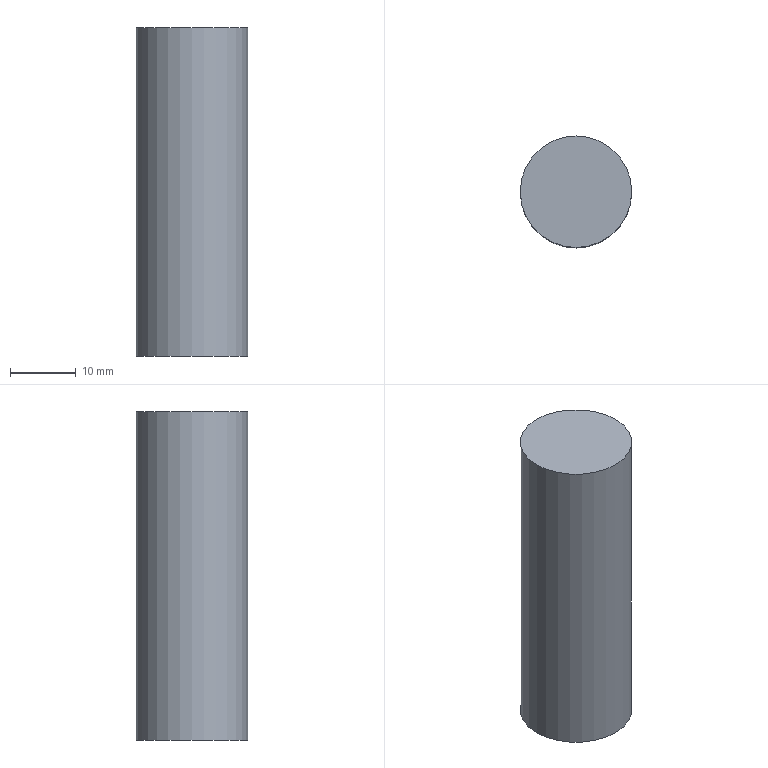Part | NX | features BREP 2 | 2 solids | 7 faces | box 17 x 17 x 50 mm | volume 12091 mm3 | plane 4 | cylinder 3 | commonest cylinder face diameters 6 x1 15 x1 17 x1
STEP:
#1=CARTESIAN_POINT('',(8.5,0.,97.));
#2=VERTEX_POINT('',#1);
#3=CARTESIAN_POINT('',(0.,0.,97.));
#4=DIRECTION('',(0.,0.,1.));
#5=DIRECTION('',(1.,0.,0.));
#6=AXIS2_PLACEMENT_3D('',#3,#4,#5);
#7=CIRCLE('',#6,8.5);
#8=EDGE_CURVE('',#2,#2,#7,.T.);
#9=ORIENTED_EDGE('',*,*,#8,.F.);
#10=EDGE_LOOP('',(#9));
#11=FACE_BOUND('',#10,.T.);
#12=CARTESIAN_POINT('',(8.5,0.,47.));
#13=VERTEX_POINT('',#12);
#14=CARTESIAN_POINT('',(0.,0.,47.));
#15=DIRECTION('',(0.,0.,1.));
#16=DIRECTION('',(1.,0.,0.));
#17=AXIS2_PLACEMENT_3D('',#14,#15,#16);
#18=CIRCLE('',#17,8.5);
#19=EDGE_CURVE('',#13,#13,#18,.T.);
#20=ORIENTED_EDGE('',*,*,#19,.T.);
#21=EDGE_LOOP('',(#20));
#22=FACE_BOUND('',#21,.T.);
#23=CARTESIAN_POINT('',(0.,0.,97.));
#24=DIRECTION('',(0.,0.,-1.));
#25=DIRECTION('',(1.,0.,0.));
#26=AXIS2_PLACEMENT_3D('',#23,#24,#25);
#27=CYLINDRICAL_SURFACE('',#26,8.5);
#28=ADVANCED_FACE('',(#11,#22),#27,.T.);
#29=ORIENTED_EDGE('',*,*,#8,.T.);
#30=EDGE_LOOP('',(#29));
#31=FACE_BOUND('',#30,.T.);
#32=CARTESIAN_POINT('',(0.,0.,97.));
#33=DIRECTION('',(0.,0.,1.));
#34=DIRECTION('',(-1.,0.,0.));
#35=AXIS2_PLACEMENT_3D('',#32,#33,#34);
#36=PLANE('',#35);
#37=ADVANCED_FACE('',(#31),#36,.T.);
#38=ORIENTED_EDGE('',*,*,#19,.F.);
#39=EDGE_LOOP('',(#38));
#40=FACE_BOUND('',#39,.T.);
#41=CARTESIAN_POINT('',(0.,0.,47.));
#42=DIRECTION('',(0.,0.,1.));
#43=DIRECTION('',(-1.,0.,0.));
#44=AXIS2_PLACEMENT_3D('',#41,#42,#43);
#45=PLANE('',#44);
#46=ADVANCED_FACE('',(#40),#45,.F.);
#47=CLOSED_SHELL('',(#28,#37,#46));
#48=MANIFOLD_SOLID_BREP('',#47);
#49=CARTESIAN_POINT('',(7.5,0.,60.));
#50=VERTEX_POINT('',#49);
#51=CARTESIAN_POINT('',(0.,0.,60.));
#52=DIRECTION('',(0.,0.,1.));
#53=DIRECTION('',(1.,0.,0.));
#54=AXIS2_PLACEMENT_3D('',#51,#52,#53);
#55=CIRCLE('',#54,7.5);
#56=EDGE_CURVE('',#50,#50,#55,.T.);
#57=ORIENTED_EDGE('',*,*,#56,.F.);
#58=EDGE_LOOP('',(#57));
#59=FACE_BOUND('',#58,.T.);
#60=CARTESIAN_POINT('',(7.5,0.,55.));
#61=VERTEX_POINT('',#60);
#62=CARTESIAN_POINT('',(0.,0.,55.));
#63=DIRECTION('',(0.,0.,1.));
#64=DIRECTION('',(1.,0.,0.));
#65=AXIS2_PLACEMENT_3D('',#62,#63,#64);
#66=CIRCLE('',#65,7.5);
#67=EDGE_CURVE('',#61,#61,#66,.T.);
#68=ORIENTED_EDGE('',*,*,#67,.T.);
#69=EDGE_LOOP('',(#68));
#70=FACE_BOUND('',#69,.T.);
#71=CARTESIAN_POINT('',(0.,0.,60.));
#72=DIRECTION('',(0.,0.,-1.));
#73=DIRECTION('',(1.,0.,0.));
#74=AXIS2_PLACEMENT_3D('',#71,#72,#73);
#75=CYLINDRICAL_SURFACE('',#74,7.5);
#76=ADVANCED_FACE('',(#59,#70),#75,.T.);
#77=CARTESIAN_POINT('',(3.,0.,60.));
#78=VERTEX_POINT('',#77);
#79=CARTESIAN_POINT('',(0.,0.,60.));
#80=DIRECTION('',(0.,0.,1.));
#81=DIRECTION('',(1.,0.,0.));
#82=AXIS2_PLACEMENT_3D('',#79,#80,#81);
#83=CIRCLE('',#82,3.);
#84=EDGE_CURVE('',#78,#78,#83,.T.);
#85=ORIENTED_EDGE('',*,*,#84,.T.);
#86=EDGE_LOOP('',(#85));
#87=FACE_BOUND('',#86,.T.);
#88=CARTESIAN_POINT('',(3.,0.,55.));
#89=VERTEX_POINT('',#88);
#90=CARTESIAN_POINT('',(0.,0.,55.));
#91=DIRECTION('',(0.,0.,1.));
#92=DIRECTION('',(1.,0.,0.));
#93=AXIS2_PLACEMENT_3D('',#90,#91,#92);
#94=CIRCLE('',#93,3.);
#95=EDGE_CURVE('',#89,#89,#94,.T.);
#96=ORIENTED_EDGE('',*,*,#95,.F.);
#97=EDGE_LOOP('',(#96));
#98=FACE_BOUND('',#97,.T.);
#99=CARTESIAN_POINT('',(0.,0.,60.));
#100=DIRECTION('',(0.,0.,-1.));
#101=DIRECTION('',(1.,0.,0.));
#102=AXIS2_PLACEMENT_3D('',#99,#100,#101);
#103=CYLINDRICAL_SURFACE('',#102,3.);
#104=ADVANCED_FACE('',(#87,#98),#103,.F.);
#105=ORIENTED_EDGE('',*,*,#56,.T.);
#106=EDGE_LOOP('',(#105));
#107=FACE_BOUND('',#106,.T.);
#108=ORIENTED_EDGE('',*,*,#84,.F.);
#109=EDGE_LOOP('',(#108));
#110=FACE_BOUND('',#109,.T.);
#111=CARTESIAN_POINT('',(0.,0.,60.));
#112=DIRECTION('',(0.,0.,1.));
#113=DIRECTION('',(-1.,0.,0.));
#114=AXIS2_PLACEMENT_3D('',#111,#112,#113);
#115=PLANE('',#114);
#116=ADVANCED_FACE('',(#107,#110),#115,.T.);
#117=ORIENTED_EDGE('',*,*,#67,.F.);
#118=EDGE_LOOP('',(#117));
#119=FACE_BOUND('',#118,.T.);
#120=ORIENTED_EDGE('',*,*,#95,.T.);
#121=EDGE_LOOP('',(#120));
#122=FACE_BOUND('',#121,.T.);
#123=CARTESIAN_POINT('',(0.,0.,55.));
#124=DIRECTION('',(0.,0.,1.));
#125=DIRECTION('',(-1.,0.,0.));
#126=AXIS2_PLACEMENT_3D('',#123,#124,#125);
#127=PLANE('',#126);
#128=ADVANCED_FACE('',(#119,#122),#127,.F.);
#129=CLOSED_SHELL('',(#76,#104,#116,#128));
#130=MANIFOLD_SOLID_BREP('',#129);
#131=(LENGTH_UNIT()NAMED_UNIT(*)SI_UNIT(.MILLI.,.METRE.));
#132=UNCERTAINTY_MEASURE_WITH_UNIT(LENGTH_MEASURE(0.00001),#131,'','');
#133=(NAMED_UNIT(*)PLANE_ANGLE_UNIT()SI_UNIT($,.RADIAN.));
#134=(NAMED_UNIT(*)SI_UNIT($,.STERADIAN.)SOLID_ANGLE_UNIT());
#135=(GEOMETRIC_REPRESENTATION_CONTEXT(3)GLOBAL_UNCERTAINTY_ASSIGNED_CONTEXT((#132))GLOBAL_UNIT_ASSIGNED_CONTEXT((#131,#133,#134))REPRESENTATION_CONTEXT('',''));
#136=ADVANCED_BREP_SHAPE_REPRESENTATION('',(#48,#130),#135);